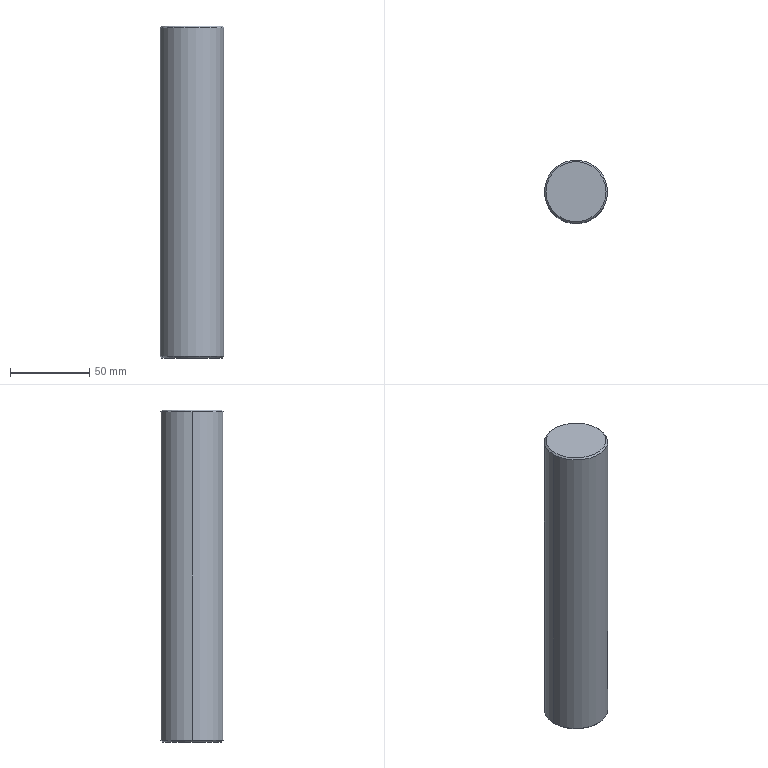Part | NX | features BREP 1 | 1 solid | 8 faces | box 40 x 40 x 210 mm | volume 263770 mm3 | cone 4 | cylinder 2 | plane 2 | commonest cylinder face diameters 40 x2
STEP:
#1=CARTESIAN_POINT('',(-19.,0.,0.));
#2=VERTEX_POINT('',#1);
#3=CARTESIAN_POINT('',(19.,0.,0.));
#4=VERTEX_POINT('',#3);
#5=CARTESIAN_POINT('',(0.,0.,0.));
#6=DIRECTION('',(0.,0.,-1.));
#7=DIRECTION('',(1.,0.,0.));
#8=AXIS2_PLACEMENT_3D('',#5,#6,#7);
#9=CIRCLE('',#8,19.);
#10=EDGE_CURVE('',#2,#4,#9,.T.);
#11=ORIENTED_EDGE('',*,*,#10,.F.);
#12=CARTESIAN_POINT('',(-20.,0.,1.));
#13=VERTEX_POINT('',#12);
#14=CARTESIAN_POINT('',(-20.,0.,1.));
#15=DIRECTION('',(-0.7071,0.,0.7071));
#16=VECTOR('',#15,1000.);
#17=LINE('',#14,#16);
#18=EDGE_CURVE('',#13,#2,#17,.F.);
#19=ORIENTED_EDGE('',*,*,#18,.F.);
#20=CARTESIAN_POINT('',(20.,0.,1.));
#21=VERTEX_POINT('',#20);
#22=CARTESIAN_POINT('',(0.,0.,1.));
#23=DIRECTION('',(0.,0.,1.));
#24=DIRECTION('',(1.,0.,0.));
#25=AXIS2_PLACEMENT_3D('',#22,#23,#24);
#26=CIRCLE('',#25,20.);
#27=EDGE_CURVE('',#21,#13,#26,.T.);
#28=ORIENTED_EDGE('',*,*,#27,.F.);
#29=CARTESIAN_POINT('',(20.,0.,1.));
#30=DIRECTION('',(0.7071,0.,0.7071));
#31=VECTOR('',#30,1000.);
#32=LINE('',#29,#31);
#33=EDGE_CURVE('',#21,#4,#32,.F.);
#34=ORIENTED_EDGE('',*,*,#33,.T.);
#35=EDGE_LOOP('',(#11,#19,#28,#34));
#36=FACE_BOUND('',#35,.T.);
#37=CARTESIAN_POINT('',(0.,0.,1.));
#38=DIRECTION('',(0.,0.,1.));
#39=DIRECTION('',(1.,0.,0.));
#40=AXIS2_PLACEMENT_3D('',#37,#38,#39);
#41=CONICAL_SURFACE('',#40,20.,0.7854);
#42=ADVANCED_FACE('',(#36),#41,.T.);
#43=CARTESIAN_POINT('',(19.,0.,210.));
#44=VERTEX_POINT('',#43);
#45=CARTESIAN_POINT('',(-19.,0.,210.));
#46=VERTEX_POINT('',#45);
#47=CARTESIAN_POINT('',(0.,0.,210.));
#48=DIRECTION('',(0.,0.,1.));
#49=DIRECTION('',(1.,0.,0.));
#50=AXIS2_PLACEMENT_3D('',#47,#48,#49);
#51=CIRCLE('',#50,19.);
#52=EDGE_CURVE('',#44,#46,#51,.T.);
#53=ORIENTED_EDGE('',*,*,#52,.F.);
#54=CARTESIAN_POINT('',(20.,0.,209.));
#55=VERTEX_POINT('',#54);
#56=CARTESIAN_POINT('',(19.,0.,210.));
#57=DIRECTION('',(0.7071,0.,-0.7071));
#58=VECTOR('',#57,1000.);
#59=LINE('',#56,#58);
#60=EDGE_CURVE('',#44,#55,#59,.T.);
#61=ORIENTED_EDGE('',*,*,#60,.T.);
#62=CARTESIAN_POINT('',(-20.,0.,209.));
#63=VERTEX_POINT('',#62);
#64=CARTESIAN_POINT('',(0.,0.,209.));
#65=DIRECTION('',(0.,0.,-1.));
#66=DIRECTION('',(1.,0.,0.));
#67=AXIS2_PLACEMENT_3D('',#64,#65,#66);
#68=CIRCLE('',#67,20.);
#69=EDGE_CURVE('',#63,#55,#68,.T.);
#70=ORIENTED_EDGE('',*,*,#69,.F.);
#71=CARTESIAN_POINT('',(-19.,0.,210.));
#72=DIRECTION('',(-0.7071,0.,-0.7071));
#73=VECTOR('',#72,1000.);
#74=LINE('',#71,#73);
#75=EDGE_CURVE('',#46,#63,#74,.T.);
#76=ORIENTED_EDGE('',*,*,#75,.F.);
#77=EDGE_LOOP('',(#53,#61,#70,#76));
#78=FACE_BOUND('',#77,.T.);
#79=CARTESIAN_POINT('',(0.,0.,210.));
#80=DIRECTION('',(0.,0.,-1.));
#81=DIRECTION('',(-1.,0.,0.));
#82=AXIS2_PLACEMENT_3D('',#79,#80,#81);
#83=CONICAL_SURFACE('',#82,19.,0.7854);
#84=ADVANCED_FACE('',(#78),#83,.T.);
#85=ORIENTED_EDGE('',*,*,#69,.T.);
#86=CARTESIAN_POINT('',(20.,0.,210.));
#87=DIRECTION('',(0.,0.,-1.));
#88=VECTOR('',#87,1000.);
#89=LINE('',#86,#88);
#90=EDGE_CURVE('',#55,#21,#89,.T.);
#91=ORIENTED_EDGE('',*,*,#90,.T.);
#92=ORIENTED_EDGE('',*,*,#27,.T.);
#93=CARTESIAN_POINT('',(-20.,0.,210.));
#94=DIRECTION('',(0.,0.,-1.));
#95=VECTOR('',#94,1000.);
#96=LINE('',#93,#95);
#97=EDGE_CURVE('',#63,#13,#96,.T.);
#98=ORIENTED_EDGE('',*,*,#97,.F.);
#99=EDGE_LOOP('',(#85,#91,#92,#98));
#100=FACE_BOUND('',#99,.T.);
#101=CARTESIAN_POINT('',(0.,0.,210.));
#102=DIRECTION('',(0.,0.,-1.));
#103=DIRECTION('',(-1.,0.,0.));
#104=AXIS2_PLACEMENT_3D('',#101,#102,#103);
#105=CYLINDRICAL_SURFACE('',#104,20.);
#106=ADVANCED_FACE('',(#100),#105,.T.);
#107=ORIENTED_EDGE('',*,*,#90,.F.);
#108=CARTESIAN_POINT('',(0.,0.,209.));
#109=DIRECTION('',(0.,0.,-1.));
#110=DIRECTION('',(1.,0.,0.));
#111=AXIS2_PLACEMENT_3D('',#108,#109,#110);
#112=CIRCLE('',#111,20.);
#113=EDGE_CURVE('',#55,#63,#112,.T.);
#114=ORIENTED_EDGE('',*,*,#113,.T.);
#115=ORIENTED_EDGE('',*,*,#97,.T.);
#116=CARTESIAN_POINT('',(0.,0.,1.));
#117=DIRECTION('',(0.,0.,1.));
#118=DIRECTION('',(1.,0.,0.));
#119=AXIS2_PLACEMENT_3D('',#116,#117,#118);
#120=CIRCLE('',#119,20.);
#121=EDGE_CURVE('',#13,#21,#120,.T.);
#122=ORIENTED_EDGE('',*,*,#121,.T.);
#123=EDGE_LOOP('',(#107,#114,#115,#122));
#124=FACE_BOUND('',#123,.T.);
#125=CARTESIAN_POINT('',(0.,0.,210.));
#126=DIRECTION('',(0.,0.,-1.));
#127=DIRECTION('',(-1.,0.,0.));
#128=AXIS2_PLACEMENT_3D('',#125,#126,#127);
#129=CYLINDRICAL_SURFACE('',#128,20.);
#130=ADVANCED_FACE('',(#124),#129,.T.);
#131=CARTESIAN_POINT('',(0.,0.,210.));
#132=DIRECTION('',(0.,0.,1.));
#133=DIRECTION('',(1.,0.,0.));
#134=AXIS2_PLACEMENT_3D('',#131,#132,#133);
#135=CIRCLE('',#134,19.);
#136=EDGE_CURVE('',#46,#44,#135,.T.);
#137=ORIENTED_EDGE('',*,*,#136,.T.);
#138=ORIENTED_EDGE('',*,*,#52,.T.);
#139=EDGE_LOOP('',(#137,#138));
#140=FACE_BOUND('',#139,.T.);
#141=CARTESIAN_POINT('',(0.,0.,210.));
#142=DIRECTION('',(0.,0.,1.));
#143=DIRECTION('',(1.,0.,0.));
#144=AXIS2_PLACEMENT_3D('',#141,#142,#143);
#145=PLANE('',#144);
#146=ADVANCED_FACE('',(#140),#145,.T.);
#147=CARTESIAN_POINT('',(0.,0.,0.));
#148=DIRECTION('',(0.,0.,-1.));
#149=DIRECTION('',(1.,0.,0.));
#150=AXIS2_PLACEMENT_3D('',#147,#148,#149);
#151=CIRCLE('',#150,19.);
#152=EDGE_CURVE('',#4,#2,#151,.T.);
#153=ORIENTED_EDGE('',*,*,#152,.T.);
#154=ORIENTED_EDGE('',*,*,#10,.T.);
#155=EDGE_LOOP('',(#153,#154));
#156=FACE_BOUND('',#155,.T.);
#157=CARTESIAN_POINT('',(0.,0.,0.));
#158=DIRECTION('',(0.,0.,1.));
#159=DIRECTION('',(1.,0.,0.));
#160=AXIS2_PLACEMENT_3D('',#157,#158,#159);
#161=PLANE('',#160);
#162=ADVANCED_FACE('',(#156),#161,.F.);
#163=ORIENTED_EDGE('',*,*,#60,.F.);
#164=ORIENTED_EDGE('',*,*,#136,.F.);
#165=ORIENTED_EDGE('',*,*,#75,.T.);
#166=ORIENTED_EDGE('',*,*,#113,.F.);
#167=EDGE_LOOP('',(#163,#164,#165,#166));
#168=FACE_BOUND('',#167,.T.);
#169=CARTESIAN_POINT('',(0.,0.,210.));
#170=DIRECTION('',(0.,0.,-1.));
#171=DIRECTION('',(-1.,0.,0.));
#172=AXIS2_PLACEMENT_3D('',#169,#170,#171);
#173=CONICAL_SURFACE('',#172,19.,0.7854);
#174=ADVANCED_FACE('',(#168),#173,.T.);
#175=ORIENTED_EDGE('',*,*,#18,.T.);
#176=ORIENTED_EDGE('',*,*,#152,.F.);
#177=ORIENTED_EDGE('',*,*,#33,.F.);
#178=ORIENTED_EDGE('',*,*,#121,.F.);
#179=EDGE_LOOP('',(#175,#176,#177,#178));
#180=FACE_BOUND('',#179,.T.);
#181=CARTESIAN_POINT('',(0.,0.,1.));
#182=DIRECTION('',(0.,0.,1.));
#183=DIRECTION('',(1.,0.,0.));
#184=AXIS2_PLACEMENT_3D('',#181,#182,#183);
#185=CONICAL_SURFACE('',#184,20.,0.7854);
#186=ADVANCED_FACE('',(#180),#185,.T.);
#187=CLOSED_SHELL('',(#42,#84,#106,#130,#146,#162,#174,#186));
#188=MANIFOLD_SOLID_BREP('',#187);
#189=(LENGTH_UNIT()NAMED_UNIT(*)SI_UNIT(.MILLI.,.METRE.));
#190=UNCERTAINTY_MEASURE_WITH_UNIT(LENGTH_MEASURE(0.00001),#189,'','');
#191=(NAMED_UNIT(*)PLANE_ANGLE_UNIT()SI_UNIT($,.RADIAN.));
#192=(NAMED_UNIT(*)SI_UNIT($,.STERADIAN.)SOLID_ANGLE_UNIT());
#193=(GEOMETRIC_REPRESENTATION_CONTEXT(3)GLOBAL_UNCERTAINTY_ASSIGNED_CONTEXT((#190))GLOBAL_UNIT_ASSIGNED_CONTEXT((#189,#191,#192))REPRESENTATION_CONTEXT('',''));
#194=ADVANCED_BREP_SHAPE_REPRESENTATION('',(#188),#193);